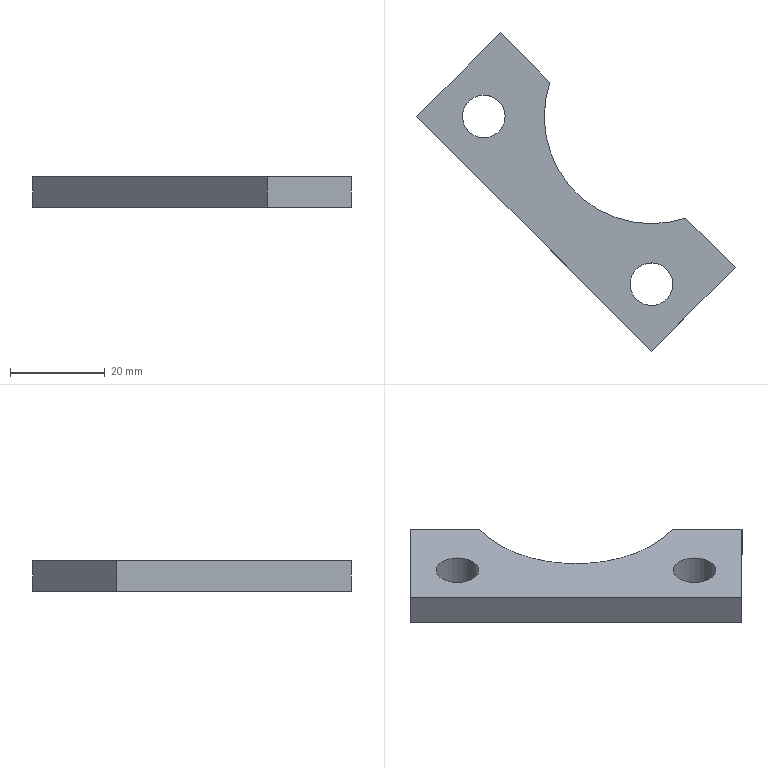Part | NX | features solid 2 | 1 solid | 10 faces | box 67.175 x 67.175 x 6.5 mm | volume 8172 mm3 | plane 7 | cylinder 3 | commonest cylinder face diameters 9 x2 45.2 x1
STEP:
#1=CARTESIAN_POINT('',(1545.796,-174.938,385.));
#2=VERTEX_POINT('',#1);
#3=CARTESIAN_POINT('',(1545.796,-174.938,378.5));
#4=VERTEX_POINT('',#3);
#5=CARTESIAN_POINT('',(1545.796,-174.938,378.5));
#6=DIRECTION('',(0.,0.,1.));
#7=VECTOR('',#6,1000.);
#8=LINE('',#5,#7);
#9=EDGE_CURVE('',#2,#4,#8,.F.);
#10=ORIENTED_EDGE('',*,*,#9,.F.);
#11=CARTESIAN_POINT('',(1556.213,-185.355,385.));
#12=VERTEX_POINT('',#11);
#13=CARTESIAN_POINT('',(1506.716,-135.858,385.));
#14=DIRECTION('',(0.7071,-0.7071,0.));
#15=VECTOR('',#14,1000.);
#16=LINE('',#13,#15);
#17=EDGE_CURVE('',#2,#12,#16,.T.);
#18=ORIENTED_EDGE('',*,*,#17,.T.);
#19=CARTESIAN_POINT('',(1556.213,-185.355,378.5));
#20=VERTEX_POINT('',#19);
#21=CARTESIAN_POINT('',(1556.213,-185.355,378.5));
#22=DIRECTION('',(0.,0.,1.));
#23=VECTOR('',#22,1000.);
#24=LINE('',#21,#23);
#25=EDGE_CURVE('',#20,#12,#24,.T.);
#26=ORIENTED_EDGE('',*,*,#25,.F.);
#27=CARTESIAN_POINT('',(1506.716,-135.858,378.5));
#28=DIRECTION('',(0.7071,-0.7071,0.));
#29=VECTOR('',#28,1000.);
#30=LINE('',#27,#29);
#31=EDGE_CURVE('',#4,#20,#30,.T.);
#32=ORIENTED_EDGE('',*,*,#31,.F.);
#33=EDGE_LOOP('',(#10,#18,#26,#32));
#34=FACE_BOUND('',#33,.T.);
#35=CARTESIAN_POINT('',(1506.716,-135.858,378.5));
#36=DIRECTION('',(-0.7071,-0.7071,0.));
#37=DIRECTION('',(-0.7071,0.7071,0.));
#38=AXIS2_PLACEMENT_3D('',#35,#36,#37);
#39=PLANE('',#38);
#40=ADVANCED_FACE('',(#34),#39,.F.);
#41=CARTESIAN_POINT('',(1517.133,-146.276,378.5));
#42=VERTEX_POINT('',#41);
#43=CARTESIAN_POINT('',(1517.133,-146.276,385.));
#44=VERTEX_POINT('',#43);
#45=CARTESIAN_POINT('',(1517.133,-146.276,378.5));
#46=DIRECTION('',(0.,0.,1.));
#47=VECTOR('',#46,1000.);
#48=LINE('',#45,#47);
#49=EDGE_CURVE('',#42,#44,#48,.T.);
#50=ORIENTED_EDGE('',*,*,#49,.F.);
#51=CARTESIAN_POINT('',(1506.716,-135.858,378.5));
#52=VERTEX_POINT('',#51);
#53=CARTESIAN_POINT('',(1506.716,-135.858,378.5));
#54=DIRECTION('',(0.7071,-0.7071,0.));
#55=VECTOR('',#54,1000.);
#56=LINE('',#53,#55);
#57=EDGE_CURVE('',#52,#42,#56,.T.);
#58=ORIENTED_EDGE('',*,*,#57,.F.);
#59=CARTESIAN_POINT('',(1506.716,-135.858,385.));
#60=VERTEX_POINT('',#59);
#61=CARTESIAN_POINT('',(1506.716,-135.858,378.5));
#62=DIRECTION('',(0.,0.,1.));
#63=VECTOR('',#62,1000.);
#64=LINE('',#61,#63);
#65=EDGE_CURVE('',#52,#60,#64,.T.);
#66=ORIENTED_EDGE('',*,*,#65,.T.);
#67=CARTESIAN_POINT('',(1506.716,-135.858,385.));
#68=DIRECTION('',(0.7071,-0.7071,0.));
#69=VECTOR('',#68,1000.);
#70=LINE('',#67,#69);
#71=EDGE_CURVE('',#60,#44,#70,.T.);
#72=ORIENTED_EDGE('',*,*,#71,.T.);
#73=EDGE_LOOP('',(#50,#58,#66,#72));
#74=FACE_BOUND('',#73,.T.);
#75=CARTESIAN_POINT('',(1506.716,-135.858,378.5));
#76=DIRECTION('',(-0.7071,-0.7071,0.));
#77=DIRECTION('',(-0.7071,0.7071,0.));
#78=AXIS2_PLACEMENT_3D('',#75,#76,#77);
#79=PLANE('',#78);
#80=ADVANCED_FACE('',(#74),#79,.F.);
#81=CARTESIAN_POINT('',(1506.362,-150.354,378.5));
#82=VERTEX_POINT('',#81);
#83=CARTESIAN_POINT('',(1503.18,-153.536,378.5));
#84=DIRECTION('',(0.,0.,1.));
#85=DIRECTION('',(0.7071,0.7071,0.));
#86=AXIS2_PLACEMENT_3D('',#83,#84,#85);
#87=CIRCLE('',#86,4.5);
#88=EDGE_CURVE('',#82,#82,#87,.T.);
#89=ORIENTED_EDGE('',*,*,#88,.T.);
#90=EDGE_LOOP('',(#89));
#91=FACE_BOUND('',#90,.T.);
#92=CARTESIAN_POINT('',(1541.718,-185.709,378.5));
#93=VERTEX_POINT('',#92);
#94=CARTESIAN_POINT('',(1538.536,-188.891,378.5));
#95=DIRECTION('',(0.,0.,-1.));
#96=DIRECTION('',(0.7071,0.7071,0.));
#97=AXIS2_PLACEMENT_3D('',#94,#95,#96);
#98=CIRCLE('',#97,4.5);
#99=EDGE_CURVE('',#93,#93,#98,.T.);
#100=ORIENTED_EDGE('',*,*,#99,.F.);
#101=EDGE_LOOP('',(#100));
#102=FACE_BOUND('',#101,.T.);
#103=CARTESIAN_POINT('',(1538.536,-153.536,378.5));
#104=DIRECTION('',(0.,0.,-1.));
#105=DIRECTION('',(-0.7071,-0.7071,0.));
#106=AXIS2_PLACEMENT_3D('',#103,#104,#105);
#107=CIRCLE('',#106,22.6);
#108=EDGE_CURVE('',#4,#42,#107,.T.);
#109=ORIENTED_EDGE('',*,*,#108,.F.);
#110=ORIENTED_EDGE('',*,*,#31,.T.);
#111=CARTESIAN_POINT('',(1538.536,-203.033,378.5));
#112=VERTEX_POINT('',#111);
#113=CARTESIAN_POINT('',(1556.213,-185.355,378.5));
#114=DIRECTION('',(-0.7071,-0.7071,0.));
#115=VECTOR('',#114,1000.);
#116=LINE('',#113,#115);
#117=EDGE_CURVE('',#20,#112,#116,.T.);
#118=ORIENTED_EDGE('',*,*,#117,.T.);
#119=CARTESIAN_POINT('',(1489.038,-153.536,378.5));
#120=VERTEX_POINT('',#119);
#121=CARTESIAN_POINT('',(1538.536,-203.033,378.5));
#122=DIRECTION('',(-0.7071,0.7071,0.));
#123=VECTOR('',#122,1000.);
#124=LINE('',#121,#123);
#125=EDGE_CURVE('',#112,#120,#124,.T.);
#126=ORIENTED_EDGE('',*,*,#125,.T.);
#127=CARTESIAN_POINT('',(1489.038,-153.536,378.5));
#128=DIRECTION('',(0.7071,0.7071,0.));
#129=VECTOR('',#128,1000.);
#130=LINE('',#127,#129);
#131=EDGE_CURVE('',#120,#52,#130,.T.);
#132=ORIENTED_EDGE('',*,*,#131,.T.);
#133=ORIENTED_EDGE('',*,*,#57,.T.);
#134=EDGE_LOOP('',(#109,#110,#118,#126,#132,#133));
#135=FACE_BOUND('',#134,.T.);
#136=CARTESIAN_POINT('',(1489.038,-153.536,378.5));
#137=DIRECTION('',(0.,0.,1.));
#138=DIRECTION('',(0.7071,0.7071,0.));
#139=AXIS2_PLACEMENT_3D('',#136,#137,#138);
#140=PLANE('',#139);
#141=ADVANCED_FACE('',(#91,#102,#135),#140,.F.);
#142=CARTESIAN_POINT('',(1506.362,-150.354,385.));
#143=VERTEX_POINT('',#142);
#144=CARTESIAN_POINT('',(1503.18,-153.536,385.));
#145=DIRECTION('',(0.,0.,1.));
#146=DIRECTION('',(0.7071,0.7071,0.));
#147=AXIS2_PLACEMENT_3D('',#144,#145,#146);
#148=CIRCLE('',#147,4.5);
#149=EDGE_CURVE('',#143,#143,#148,.T.);
#150=ORIENTED_EDGE('',*,*,#149,.F.);
#151=EDGE_LOOP('',(#150));
#152=FACE_BOUND('',#151,.T.);
#153=CARTESIAN_POINT('',(1541.718,-185.709,385.));
#154=VERTEX_POINT('',#153);
#155=CARTESIAN_POINT('',(1538.536,-188.891,385.));
#156=DIRECTION('',(0.,0.,-1.));
#157=DIRECTION('',(0.7071,0.7071,0.));
#158=AXIS2_PLACEMENT_3D('',#155,#156,#157);
#159=CIRCLE('',#158,4.5);
#160=EDGE_CURVE('',#154,#154,#159,.T.);
#161=ORIENTED_EDGE('',*,*,#160,.T.);
#162=EDGE_LOOP('',(#161));
#163=FACE_BOUND('',#162,.T.);
#164=ORIENTED_EDGE('',*,*,#17,.F.);
#165=CARTESIAN_POINT('',(1538.536,-153.536,385.));
#166=DIRECTION('',(0.,0.,-1.));
#167=DIRECTION('',(-0.7071,-0.7071,0.));
#168=AXIS2_PLACEMENT_3D('',#165,#166,#167);
#169=CIRCLE('',#168,22.6);
#170=EDGE_CURVE('',#2,#44,#169,.T.);
#171=ORIENTED_EDGE('',*,*,#170,.T.);
#172=ORIENTED_EDGE('',*,*,#71,.F.);
#173=CARTESIAN_POINT('',(1489.038,-153.536,385.));
#174=VERTEX_POINT('',#173);
#175=CARTESIAN_POINT('',(1489.038,-153.536,385.));
#176=DIRECTION('',(0.7071,0.7071,0.));
#177=VECTOR('',#176,1000.);
#178=LINE('',#175,#177);
#179=EDGE_CURVE('',#174,#60,#178,.T.);
#180=ORIENTED_EDGE('',*,*,#179,.F.);
#181=CARTESIAN_POINT('',(1538.536,-203.033,385.));
#182=VERTEX_POINT('',#181);
#183=CARTESIAN_POINT('',(1538.536,-203.033,385.));
#184=DIRECTION('',(-0.7071,0.7071,0.));
#185=VECTOR('',#184,1000.);
#186=LINE('',#183,#185);
#187=EDGE_CURVE('',#182,#174,#186,.T.);
#188=ORIENTED_EDGE('',*,*,#187,.F.);
#189=CARTESIAN_POINT('',(1556.213,-185.355,385.));
#190=DIRECTION('',(-0.7071,-0.7071,0.));
#191=VECTOR('',#190,1000.);
#192=LINE('',#189,#191);
#193=EDGE_CURVE('',#12,#182,#192,.T.);
#194=ORIENTED_EDGE('',*,*,#193,.F.);
#195=EDGE_LOOP('',(#164,#171,#172,#180,#188,#194));
#196=FACE_BOUND('',#195,.T.);
#197=CARTESIAN_POINT('',(1489.038,-153.536,385.));
#198=DIRECTION('',(0.,0.,1.));
#199=DIRECTION('',(0.7071,0.7071,0.));
#200=AXIS2_PLACEMENT_3D('',#197,#198,#199);
#201=PLANE('',#200);
#202=ADVANCED_FACE('',(#152,#163,#196),#201,.T.);
#203=ORIENTED_EDGE('',*,*,#179,.T.);
#204=ORIENTED_EDGE('',*,*,#65,.F.);
#205=ORIENTED_EDGE('',*,*,#131,.F.);
#206=CARTESIAN_POINT('',(1489.038,-153.536,378.5));
#207=DIRECTION('',(0.,0.,1.));
#208=VECTOR('',#207,1000.);
#209=LINE('',#206,#208);
#210=EDGE_CURVE('',#120,#174,#209,.T.);
#211=ORIENTED_EDGE('',*,*,#210,.T.);
#212=EDGE_LOOP('',(#203,#204,#205,#211));
#213=FACE_BOUND('',#212,.T.);
#214=CARTESIAN_POINT('',(1489.038,-153.536,378.5));
#215=DIRECTION('',(0.7071,-0.7071,0.));
#216=DIRECTION('',(0.,0.,1.));
#217=AXIS2_PLACEMENT_3D('',#214,#215,#216);
#218=PLANE('',#217);
#219=ADVANCED_FACE('',(#213),#218,.F.);
#220=ORIENTED_EDGE('',*,*,#193,.T.);
#221=CARTESIAN_POINT('',(1538.536,-203.033,378.5));
#222=DIRECTION('',(0.,0.,1.));
#223=VECTOR('',#222,1000.);
#224=LINE('',#221,#223);
#225=EDGE_CURVE('',#112,#182,#224,.T.);
#226=ORIENTED_EDGE('',*,*,#225,.F.);
#227=ORIENTED_EDGE('',*,*,#117,.F.);
#228=ORIENTED_EDGE('',*,*,#25,.T.);
#229=EDGE_LOOP('',(#220,#226,#227,#228));
#230=FACE_BOUND('',#229,.T.);
#231=CARTESIAN_POINT('',(1556.213,-185.355,378.5));
#232=DIRECTION('',(-0.7071,0.7071,0.));
#233=DIRECTION('',(0.7071,0.7071,0.));
#234=AXIS2_PLACEMENT_3D('',#231,#232,#233);
#235=PLANE('',#234);
#236=ADVANCED_FACE('',(#230),#235,.F.);
#237=ORIENTED_EDGE('',*,*,#99,.T.);
#238=EDGE_LOOP('',(#237));
#239=FACE_BOUND('',#238,.T.);
#240=ORIENTED_EDGE('',*,*,#160,.F.);
#241=EDGE_LOOP('',(#240));
#242=FACE_BOUND('',#241,.T.);
#243=CARTESIAN_POINT('',(1538.536,-188.891,378.5));
#244=DIRECTION('',(0.,0.,1.));
#245=DIRECTION('',(0.7071,0.7071,0.));
#246=AXIS2_PLACEMENT_3D('',#243,#244,#245);
#247=CYLINDRICAL_SURFACE('',#246,4.5);
#248=ADVANCED_FACE('',(#239,#242),#247,.F.);
#249=ORIENTED_EDGE('',*,*,#187,.T.);
#250=ORIENTED_EDGE('',*,*,#210,.F.);
#251=ORIENTED_EDGE('',*,*,#125,.F.);
#252=ORIENTED_EDGE('',*,*,#225,.T.);
#253=EDGE_LOOP('',(#249,#250,#251,#252));
#254=FACE_BOUND('',#253,.T.);
#255=CARTESIAN_POINT('',(1538.536,-203.033,378.5));
#256=DIRECTION('',(0.7071,0.7071,0.));
#257=DIRECTION('',(0.7071,-0.7071,0.));
#258=AXIS2_PLACEMENT_3D('',#255,#256,#257);
#259=PLANE('',#258);
#260=ADVANCED_FACE('',(#254),#259,.F.);
#261=ORIENTED_EDGE('',*,*,#88,.F.);
#262=EDGE_LOOP('',(#261));
#263=FACE_BOUND('',#262,.T.);
#264=ORIENTED_EDGE('',*,*,#149,.T.);
#265=EDGE_LOOP('',(#264));
#266=FACE_BOUND('',#265,.T.);
#267=CARTESIAN_POINT('',(1503.18,-153.536,378.5));
#268=DIRECTION('',(0.,0.,1.));
#269=DIRECTION('',(0.7071,0.7071,0.));
#270=AXIS2_PLACEMENT_3D('',#267,#268,#269);
#271=CYLINDRICAL_SURFACE('',#270,4.5);
#272=ADVANCED_FACE('',(#263,#266),#271,.F.);
#273=ORIENTED_EDGE('',*,*,#9,.T.);
#274=ORIENTED_EDGE('',*,*,#108,.T.);
#275=ORIENTED_EDGE('',*,*,#49,.T.);
#276=ORIENTED_EDGE('',*,*,#170,.F.);
#277=EDGE_LOOP('',(#273,#274,#275,#276));
#278=FACE_BOUND('',#277,.T.);
#279=CARTESIAN_POINT('',(1538.536,-153.536,378.5));
#280=DIRECTION('',(0.,0.,1.));
#281=DIRECTION('',(0.7071,0.7071,0.));
#282=AXIS2_PLACEMENT_3D('',#279,#280,#281);
#283=CYLINDRICAL_SURFACE('',#282,22.6);
#284=ADVANCED_FACE('',(#278),#283,.F.);
#285=CLOSED_SHELL('',(#40,#80,#141,#202,#219,#236,#248,#260,#272,#284));
#286=MANIFOLD_SOLID_BREP('',#285);
#287=(LENGTH_UNIT()NAMED_UNIT(*)SI_UNIT(.MILLI.,.METRE.));
#288=UNCERTAINTY_MEASURE_WITH_UNIT(LENGTH_MEASURE(0.00001),#287,'','');
#289=(NAMED_UNIT(*)PLANE_ANGLE_UNIT()SI_UNIT($,.RADIAN.));
#290=(NAMED_UNIT(*)SI_UNIT($,.STERADIAN.)SOLID_ANGLE_UNIT());
#291=(GEOMETRIC_REPRESENTATION_CONTEXT(3)GLOBAL_UNCERTAINTY_ASSIGNED_CONTEXT((#288))GLOBAL_UNIT_ASSIGNED_CONTEXT((#287,#289,#290))REPRESENTATION_CONTEXT('',''));
#292=ADVANCED_BREP_SHAPE_REPRESENTATION('',(#286),#291);